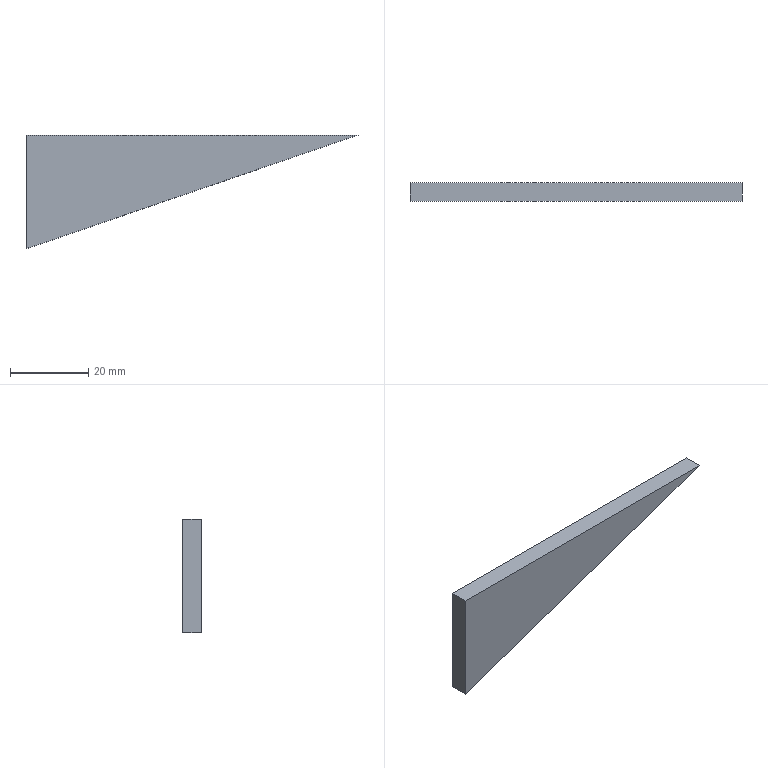Part | NX | features BREP 1 | 1 solid | 5 faces | box 85.09 x 4.775 x 29.21 mm | volume 5934 mm3 | plane 5
STEP:
#1=CARTESIAN_POINT('',(85.09,0.,0.));
#2=VERTEX_POINT('',#1);
#3=CARTESIAN_POINT('',(0.,0.,-29.21));
#4=VERTEX_POINT('',#3);
#5=CARTESIAN_POINT('',(85.09,0.,0.));
#6=DIRECTION('',(-0.9458,0.,-0.3247));
#7=VECTOR('',#6,1000.);
#8=LINE('',#5,#7);
#9=EDGE_CURVE('',#2,#4,#8,.T.);
#10=ORIENTED_EDGE('',*,*,#9,.T.);
#11=CARTESIAN_POINT('',(0.,0.,0.));
#12=VERTEX_POINT('',#11);
#13=CARTESIAN_POINT('',(0.,0.,-29.21));
#14=DIRECTION('',(0.,0.,1.));
#15=VECTOR('',#14,1000.);
#16=LINE('',#13,#15);
#17=EDGE_CURVE('',#4,#12,#16,.T.);
#18=ORIENTED_EDGE('',*,*,#17,.T.);
#19=CARTESIAN_POINT('',(0.,0.,0.));
#20=DIRECTION('',(1.,0.,0.));
#21=VECTOR('',#20,1000.);
#22=LINE('',#19,#21);
#23=EDGE_CURVE('',#12,#2,#22,.T.);
#24=ORIENTED_EDGE('',*,*,#23,.T.);
#25=EDGE_LOOP('',(#10,#18,#24));
#26=FACE_BOUND('',#25,.T.);
#27=CARTESIAN_POINT('',(0.,0.,0.));
#28=DIRECTION('',(0.,1.,0.));
#29=DIRECTION('',(1.,0.,0.));
#30=AXIS2_PLACEMENT_3D('',#27,#28,#29);
#31=PLANE('',#30);
#32=ADVANCED_FACE('',(#26),#31,.T.);
#33=CARTESIAN_POINT('',(0.,-4.775,0.));
#34=VERTEX_POINT('',#33);
#35=CARTESIAN_POINT('',(0.,0.,0.));
#36=DIRECTION('',(0.,-1.,0.));
#37=VECTOR('',#36,1000.);
#38=LINE('',#35,#37);
#39=EDGE_CURVE('',#12,#34,#38,.T.);
#40=ORIENTED_EDGE('',*,*,#39,.T.);
#41=CARTESIAN_POINT('',(85.09,-4.775,0.));
#42=VERTEX_POINT('',#41);
#43=CARTESIAN_POINT('',(0.,-4.775,0.));
#44=DIRECTION('',(1.,0.,0.));
#45=VECTOR('',#44,1000.);
#46=LINE('',#43,#45);
#47=EDGE_CURVE('',#34,#42,#46,.T.);
#48=ORIENTED_EDGE('',*,*,#47,.T.);
#49=CARTESIAN_POINT('',(85.09,0.,0.));
#50=DIRECTION('',(0.,-1.,0.));
#51=VECTOR('',#50,1000.);
#52=LINE('',#49,#51);
#53=EDGE_CURVE('',#2,#42,#52,.T.);
#54=ORIENTED_EDGE('',*,*,#53,.F.);
#55=ORIENTED_EDGE('',*,*,#23,.F.);
#56=EDGE_LOOP('',(#40,#48,#54,#55));
#57=FACE_BOUND('',#56,.T.);
#58=CARTESIAN_POINT('',(42.545,-2.388,0.));
#59=DIRECTION('',(0.,0.,1.));
#60=DIRECTION('',(1.,0.,0.));
#61=AXIS2_PLACEMENT_3D('',#58,#59,#60);
#62=PLANE('',#61);
#63=ADVANCED_FACE('',(#57),#62,.T.);
#64=ORIENTED_EDGE('',*,*,#53,.T.);
#65=CARTESIAN_POINT('',(0.,-4.775,-29.21));
#66=VERTEX_POINT('',#65);
#67=CARTESIAN_POINT('',(85.09,-4.775,0.));
#68=DIRECTION('',(-0.9458,0.,-0.3247));
#69=VECTOR('',#68,1000.);
#70=LINE('',#67,#69);
#71=EDGE_CURVE('',#42,#66,#70,.T.);
#72=ORIENTED_EDGE('',*,*,#71,.T.);
#73=CARTESIAN_POINT('',(0.,0.,-29.21));
#74=DIRECTION('',(0.,-1.,0.));
#75=VECTOR('',#74,1000.);
#76=LINE('',#73,#75);
#77=EDGE_CURVE('',#4,#66,#76,.T.);
#78=ORIENTED_EDGE('',*,*,#77,.F.);
#79=ORIENTED_EDGE('',*,*,#9,.F.);
#80=EDGE_LOOP('',(#64,#72,#78,#79));
#81=FACE_BOUND('',#80,.T.);
#82=CARTESIAN_POINT('',(42.545,-2.388,-14.605));
#83=DIRECTION('',(0.3247,0.,-0.9458));
#84=DIRECTION('',(0.,-1.,0.));
#85=AXIS2_PLACEMENT_3D('',#82,#83,#84);
#86=PLANE('',#85);
#87=ADVANCED_FACE('',(#81),#86,.T.);
#88=ORIENTED_EDGE('',*,*,#77,.T.);
#89=CARTESIAN_POINT('',(0.,-4.775,-29.21));
#90=DIRECTION('',(0.,0.,1.));
#91=VECTOR('',#90,1000.);
#92=LINE('',#89,#91);
#93=EDGE_CURVE('',#66,#34,#92,.T.);
#94=ORIENTED_EDGE('',*,*,#93,.T.);
#95=ORIENTED_EDGE('',*,*,#39,.F.);
#96=ORIENTED_EDGE('',*,*,#17,.F.);
#97=EDGE_LOOP('',(#88,#94,#95,#96));
#98=FACE_BOUND('',#97,.T.);
#99=CARTESIAN_POINT('',(0.,-2.388,-14.605));
#100=DIRECTION('',(-1.,0.,0.));
#101=DIRECTION('',(0.,0.,1.));
#102=AXIS2_PLACEMENT_3D('',#99,#100,#101);
#103=PLANE('',#102);
#104=ADVANCED_FACE('',(#98),#103,.T.);
#105=ORIENTED_EDGE('',*,*,#93,.F.);
#106=ORIENTED_EDGE('',*,*,#71,.F.);
#107=ORIENTED_EDGE('',*,*,#47,.F.);
#108=EDGE_LOOP('',(#105,#106,#107));
#109=FACE_BOUND('',#108,.T.);
#110=CARTESIAN_POINT('',(0.,-4.775,0.));
#111=DIRECTION('',(0.,1.,0.));
#112=DIRECTION('',(1.,0.,0.));
#113=AXIS2_PLACEMENT_3D('',#110,#111,#112);
#114=PLANE('',#113);
#115=ADVANCED_FACE('',(#109),#114,.F.);
#116=CLOSED_SHELL('',(#32,#63,#87,#104,#115));
#117=MANIFOLD_SOLID_BREP('',#116);
#118=(LENGTH_UNIT()NAMED_UNIT(*)SI_UNIT(.MILLI.,.METRE.));
#119=UNCERTAINTY_MEASURE_WITH_UNIT(LENGTH_MEASURE(0.00001),#118,'','');
#120=(NAMED_UNIT(*)PLANE_ANGLE_UNIT()SI_UNIT($,.RADIAN.));
#121=(NAMED_UNIT(*)SI_UNIT($,.STERADIAN.)SOLID_ANGLE_UNIT());
#122=(GEOMETRIC_REPRESENTATION_CONTEXT(3)GLOBAL_UNCERTAINTY_ASSIGNED_CONTEXT((#119))GLOBAL_UNIT_ASSIGNED_CONTEXT((#118,#120,#121))REPRESENTATION_CONTEXT('',''));
#123=ADVANCED_BREP_SHAPE_REPRESENTATION('',(#117),#122);